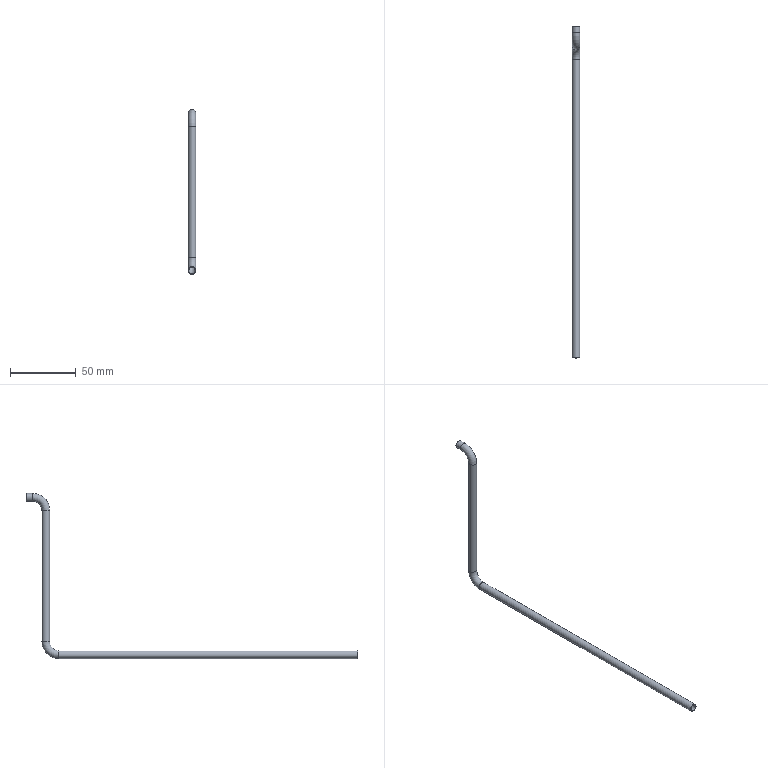Part | STEP file | 1-74 | 1 solid | 12 faces | box 6 x 253 x 126 mm | volume 3148 mm3 | cylinder 6 | torus 4 | plane 2 | commonest cylinder face diameters 5 x3 6 x3
STEP:
#1=CARTESIAN_POINT('',(0.,0.,0.));
#2=DIRECTION('',(0.,0.,1.));
#3=DIRECTION('',(1.,0.,0.));
#4=AXIS2_PLACEMENT_3D('',#1,#2,#3);
#5=CARTESIAN_POINT('',(3.,0.,0.));
#6=VERTEX_POINT('',#5);
#7=CARTESIAN_POINT('',(0.,0.,0.));
#8=DIRECTION('',(0.,-1.,0.));
#9=DIRECTION('',(1.,0.,0.));
#10=AXIS2_PLACEMENT_3D('',#7,#8,#9);
#11=CIRCLE('',#10,3.);
#12=CARTESIAN_POINT('',(0.,0.,0.));
#13=DIRECTION('',(0.,1.,0.));
#14=DIRECTION('',(1.,0.,0.));
#15=AXIS2_PLACEMENT_3D('',#12,#13,#14);
#16=CYLINDRICAL_SURFACE('',#15,3.);
#17=CARTESIAN_POINT('',(6.283,0.));
#18=DIRECTION('',(-1.,0.));
#19=VECTOR('',#18,1.);
#20=LINE('',#17,#19);
#21=(GEOMETRIC_REPRESENTATION_CONTEXT(2)PARAMETRIC_REPRESENTATION_CONTEXT()REPRESENTATION_CONTEXT('',''));
#22=DEFINITIONAL_REPRESENTATION('',(#20),#21);
#23=PCURVE('',#16,#22);
#24=CARTESIAN_POINT('',(0.,0.,0.));
#25=DIRECTION('',(0.,-1.,0.));
#26=DIRECTION('',(1.,0.,0.));
#27=AXIS2_PLACEMENT_3D('',#24,#25,#26);
#28=PLANE('',#27);
#29=CARTESIAN_POINT('',(0.,0.));
#30=DIRECTION('',(1.,0.));
#31=AXIS2_PLACEMENT_2D('',#29,#30);
#32=CIRCLE('',#31,3.);
#33=(GEOMETRIC_REPRESENTATION_CONTEXT(2)PARAMETRIC_REPRESENTATION_CONTEXT()REPRESENTATION_CONTEXT('',''));
#34=DEFINITIONAL_REPRESENTATION('',(#32),#33);
#35=PCURVE('',#28,#34);
#36=SURFACE_CURVE('',#11,(#23,#35),.PCURVE_S1.);
#37=EDGE_CURVE('',#6,#6,#36,.T.);
#38=ORIENTED_EDGE('',*,*,#37,.F.);
#39=CARTESIAN_POINT('',(3.,228.,0.));
#40=VERTEX_POINT('',#39);
#41=CARTESIAN_POINT('',(3.,0.,0.));
#42=DIRECTION('',(0.,1.,0.));
#43=VECTOR('',#42,1.);
#44=LINE('',#41,#43);
#45=CARTESIAN_POINT('',(6.283,0.));
#46=DIRECTION('',(0.,1.));
#47=VECTOR('',#46,1.);
#48=LINE('',#45,#47);
#49=(GEOMETRIC_REPRESENTATION_CONTEXT(2)PARAMETRIC_REPRESENTATION_CONTEXT()REPRESENTATION_CONTEXT('',''));
#50=DEFINITIONAL_REPRESENTATION('',(#48),#49);
#51=PCURVE('',#16,#50);
#52=CARTESIAN_POINT('',(0.,0.));
#53=DIRECTION('',(0.,1.));
#54=VECTOR('',#53,1.);
#55=LINE('',#52,#54);
#56=(GEOMETRIC_REPRESENTATION_CONTEXT(2)PARAMETRIC_REPRESENTATION_CONTEXT()REPRESENTATION_CONTEXT('',''));
#57=DEFINITIONAL_REPRESENTATION('',(#55),#56);
#58=PCURVE('',#16,#57);
#59=SEAM_CURVE('',#44,(#51,#58),.PCURVE_S1.);
#60=EDGE_CURVE('',#6,#40,#59,.T.);
#61=ORIENTED_EDGE('',*,*,#60,.T.);
#62=CARTESIAN_POINT('',(-3.,228.,0.));
#63=VERTEX_POINT('',#62);
#64=CARTESIAN_POINT('',(0.,228.,0.));
#65=DIRECTION('',(0.,1.,0.));
#66=DIRECTION('',(-1.,0.,0.));
#67=AXIS2_PLACEMENT_3D('',#64,#65,#66);
#68=CIRCLE('',#67,3.);
#69=CARTESIAN_POINT('',(3.142,228.));
#70=DIRECTION('',(1.,0.));
#71=VECTOR('',#70,1.);
#72=LINE('',#69,#71);
#73=(GEOMETRIC_REPRESENTATION_CONTEXT(2)PARAMETRIC_REPRESENTATION_CONTEXT()REPRESENTATION_CONTEXT('',''));
#74=DEFINITIONAL_REPRESENTATION('',(#72),#73);
#75=PCURVE('',#16,#74);
#76=CARTESIAN_POINT('',(0.,228.,10.));
#77=DIRECTION('',(-1.,0.,0.));
#78=DIRECTION('',(0.,0.,-1.));
#79=AXIS2_PLACEMENT_3D('',#76,#77,#78);
#80=TOROIDAL_SURFACE('',#79,10.,3.);
#81=CARTESIAN_POINT('',(6.283,1.571));
#82=CARTESIAN_POINT('',(6.283,1.618));
#83=CARTESIAN_POINT('',(6.283,1.714));
#84=CARTESIAN_POINT('',(6.283,1.856));
#85=CARTESIAN_POINT('',(6.283,1.999));
#86=CARTESIAN_POINT('',(6.283,2.142));
#87=CARTESIAN_POINT('',(6.283,2.285));
#88=CARTESIAN_POINT('',(6.283,2.428));
#89=CARTESIAN_POINT('',(6.283,2.57));
#90=CARTESIAN_POINT('',(6.283,2.713));
#91=CARTESIAN_POINT('',(6.283,2.856));
#92=CARTESIAN_POINT('',(6.283,2.999));
#93=CARTESIAN_POINT('',(6.283,3.142));
#94=CARTESIAN_POINT('',(6.283,3.284));
#95=CARTESIAN_POINT('',(6.283,3.427));
#96=CARTESIAN_POINT('',(6.283,3.57));
#97=CARTESIAN_POINT('',(6.283,3.713));
#98=CARTESIAN_POINT('',(6.283,3.856));
#99=CARTESIAN_POINT('',(6.283,3.998));
#100=CARTESIAN_POINT('',(6.283,4.141));
#101=CARTESIAN_POINT('',(6.283,4.284));
#102=CARTESIAN_POINT('',(6.283,4.427));
#103=CARTESIAN_POINT('',(6.283,4.57));
#104=CARTESIAN_POINT('',(6.283,4.665));
#105=CARTESIAN_POINT('',(6.283,4.712));
#106=B_SPLINE_CURVE_WITH_KNOTS('',3,(#81,#82,#83,#84,#85,#86,#87,#88,#89,#90,#91,#92,#93,#94,#95,#96,#97,#98,#99,#100,#101,#102,#103,#104,#105),.UNSPECIFIED.,.F.,.F.,(4,1,1,1,1,1,1,1,1,1,1,1,1,1,1,1,1,1,1,1,1,1,4),(0.,0.1428,0.2856,0.4284,0.5712,0.714,0.8568,0.9996,1.142,1.285,1.428,1.571,1.714,1.856,1.999,2.142,2.285,2.428,2.57,2.713,2.856,2.999,3.142),.QUASI_UNIFORM_KNOTS.);
#107=(GEOMETRIC_REPRESENTATION_CONTEXT(2)PARAMETRIC_REPRESENTATION_CONTEXT()REPRESENTATION_CONTEXT('',''));
#108=DEFINITIONAL_REPRESENTATION('',(#106),#107);
#109=PCURVE('',#80,#108);
#110=SURFACE_CURVE('',#68,(#75,#109),.PCURVE_S1.);
#111=EDGE_CURVE('',#63,#40,#110,.T.);
#112=ORIENTED_EDGE('',*,*,#111,.F.);
#113=CARTESIAN_POINT('',(0.,228.,0.));
#114=DIRECTION('',(0.,1.,0.));
#115=DIRECTION('',(1.,0.,0.));
#116=AXIS2_PLACEMENT_3D('',#113,#114,#115);
#117=CIRCLE('',#116,3.);
#118=CARTESIAN_POINT('',(0.,228.));
#119=DIRECTION('',(1.,0.));
#120=VECTOR('',#119,1.);
#121=LINE('',#118,#120);
#122=(GEOMETRIC_REPRESENTATION_CONTEXT(2)PARAMETRIC_REPRESENTATION_CONTEXT()REPRESENTATION_CONTEXT('',''));
#123=DEFINITIONAL_REPRESENTATION('',(#121),#122);
#124=PCURVE('',#16,#123);
#125=CARTESIAN_POINT('',(6.283,4.712));
#126=DIRECTION('',(0.,1.));
#127=VECTOR('',#126,1.);
#128=LINE('',#125,#127);
#129=(GEOMETRIC_REPRESENTATION_CONTEXT(2)PARAMETRIC_REPRESENTATION_CONTEXT()REPRESENTATION_CONTEXT('',''));
#130=DEFINITIONAL_REPRESENTATION('',(#128),#129);
#131=PCURVE('',#80,#130);
#132=SURFACE_CURVE('',#117,(#124,#131),.PCURVE_S1.);
#133=EDGE_CURVE('',#40,#63,#132,.T.);
#134=ORIENTED_EDGE('',*,*,#133,.F.);
#135=ORIENTED_EDGE('',*,*,#60,.F.);
#136=EDGE_LOOP('',(#38,#61,#112,#134,#135));
#137=FACE_BOUND('',#136,.T.);
#138=ADVANCED_FACE('',(#137),#16,.T.);
#139=ORIENTED_EDGE('',*,*,#111,.T.);
#140=ORIENTED_EDGE('',*,*,#133,.T.);
#141=CARTESIAN_POINT('',(-3.,238.,10.));
#142=VERTEX_POINT('',#141);
#143=CARTESIAN_POINT('',(-3.,228.,10.));
#144=DIRECTION('',(1.,0.,0.));
#145=DIRECTION('',(0.,0.,-1.));
#146=AXIS2_PLACEMENT_3D('',#143,#144,#145);
#147=CIRCLE('',#146,10.);
#148=CARTESIAN_POINT('',(6.283,7.854));
#149=DIRECTION('',(-1.,0.));
#150=VECTOR('',#149,1.);
#151=LINE('',#148,#150);
#152=(GEOMETRIC_REPRESENTATION_CONTEXT(2)PARAMETRIC_REPRESENTATION_CONTEXT()REPRESENTATION_CONTEXT('',''));
#153=DEFINITIONAL_REPRESENTATION('',(#151),#152);
#154=PCURVE('',#80,#153);
#155=CARTESIAN_POINT('',(6.283,1.571));
#156=DIRECTION('',(-1.,0.));
#157=VECTOR('',#156,1.);
#158=LINE('',#155,#157);
#159=(GEOMETRIC_REPRESENTATION_CONTEXT(2)PARAMETRIC_REPRESENTATION_CONTEXT()REPRESENTATION_CONTEXT('',''));
#160=DEFINITIONAL_REPRESENTATION('',(#158),#159);
#161=PCURVE('',#80,#160);
#162=SEAM_CURVE('',#147,(#154,#161),.PCURVE_S1.);
#163=EDGE_CURVE('',#63,#142,#162,.T.);
#164=ORIENTED_EDGE('',*,*,#163,.T.);
#165=CARTESIAN_POINT('',(3.,238.,10.));
#166=VERTEX_POINT('',#165);
#167=CARTESIAN_POINT('',(0.,238.,10.));
#168=DIRECTION('',(0.,0.,-1.));
#169=DIRECTION('',(-1.,0.,0.));
#170=AXIS2_PLACEMENT_3D('',#167,#168,#169);
#171=CIRCLE('',#170,3.);
#172=CARTESIAN_POINT('',(4.712,7.854));
#173=DIRECTION('',(0.,-1.));
#174=VECTOR('',#173,1.);
#175=LINE('',#172,#174);
#176=(GEOMETRIC_REPRESENTATION_CONTEXT(2)PARAMETRIC_REPRESENTATION_CONTEXT()REPRESENTATION_CONTEXT('',''));
#177=DEFINITIONAL_REPRESENTATION('',(#175),#176);
#178=PCURVE('',#80,#177);
#179=CARTESIAN_POINT('',(0.,238.,10.));
#180=DIRECTION('',(0.,0.,1.));
#181=DIRECTION('',(1.,0.,0.));
#182=AXIS2_PLACEMENT_3D('',#179,#180,#181);
#183=CYLINDRICAL_SURFACE('',#182,3.);
#184=CARTESIAN_POINT('',(3.142,0.));
#185=DIRECTION('',(-1.,0.));
#186=VECTOR('',#185,1.);
#187=LINE('',#184,#186);
#188=(GEOMETRIC_REPRESENTATION_CONTEXT(2)PARAMETRIC_REPRESENTATION_CONTEXT()REPRESENTATION_CONTEXT('',''));
#189=DEFINITIONAL_REPRESENTATION('',(#187),#188);
#190=PCURVE('',#183,#189);
#191=SURFACE_CURVE('',#171,(#178,#190),.PCURVE_S1.);
#192=EDGE_CURVE('',#142,#166,#191,.T.);
#193=ORIENTED_EDGE('',*,*,#192,.T.);
#194=CARTESIAN_POINT('',(0.,238.,10.));
#195=DIRECTION('',(0.,0.,-1.));
#196=DIRECTION('',(1.,0.,0.));
#197=AXIS2_PLACEMENT_3D('',#194,#195,#196);
#198=CIRCLE('',#197,3.);
#199=CARTESIAN_POINT('',(4.712,4.712));
#200=DIRECTION('',(0.,-1.));
#201=VECTOR('',#200,1.);
#202=LINE('',#199,#201);
#203=(GEOMETRIC_REPRESENTATION_CONTEXT(2)PARAMETRIC_REPRESENTATION_CONTEXT()REPRESENTATION_CONTEXT('',''));
#204=DEFINITIONAL_REPRESENTATION('',(#202),#203);
#205=PCURVE('',#80,#204);
#206=CARTESIAN_POINT('',(6.283,0.));
#207=DIRECTION('',(-1.,0.));
#208=VECTOR('',#207,1.);
#209=LINE('',#206,#208);
#210=(GEOMETRIC_REPRESENTATION_CONTEXT(2)PARAMETRIC_REPRESENTATION_CONTEXT()REPRESENTATION_CONTEXT('',''));
#211=DEFINITIONAL_REPRESENTATION('',(#209),#210);
#212=PCURVE('',#183,#211);
#213=SURFACE_CURVE('',#198,(#205,#212),.PCURVE_S1.);
#214=EDGE_CURVE('',#166,#142,#213,.T.);
#215=ORIENTED_EDGE('',*,*,#214,.T.);
#216=ORIENTED_EDGE('',*,*,#163,.F.);
#217=EDGE_LOOP('',(#139,#140,#164,#193,#215,#216));
#218=FACE_BOUND('',#217,.T.);
#219=ADVANCED_FACE('',(#218),#80,.T.);
#220=ORIENTED_EDGE('',*,*,#192,.F.);
#221=ORIENTED_EDGE('',*,*,#214,.F.);
#222=CARTESIAN_POINT('',(3.,238.,110.));
#223=VERTEX_POINT('',#222);
#224=CARTESIAN_POINT('',(3.,238.,10.));
#225=DIRECTION('',(0.,0.,1.));
#226=VECTOR('',#225,1.);
#227=LINE('',#224,#226);
#228=CARTESIAN_POINT('',(6.283,0.));
#229=DIRECTION('',(0.,1.));
#230=VECTOR('',#229,1.);
#231=LINE('',#228,#230);
#232=(GEOMETRIC_REPRESENTATION_CONTEXT(2)PARAMETRIC_REPRESENTATION_CONTEXT()REPRESENTATION_CONTEXT('',''));
#233=DEFINITIONAL_REPRESENTATION('',(#231),#232);
#234=PCURVE('',#183,#233);
#235=CARTESIAN_POINT('',(0.,0.));
#236=DIRECTION('',(0.,1.));
#237=VECTOR('',#236,1.);
#238=LINE('',#235,#237);
#239=(GEOMETRIC_REPRESENTATION_CONTEXT(2)PARAMETRIC_REPRESENTATION_CONTEXT()REPRESENTATION_CONTEXT('',''));
#240=DEFINITIONAL_REPRESENTATION('',(#238),#239);
#241=PCURVE('',#183,#240);
#242=SEAM_CURVE('',#227,(#234,#241),.PCURVE_S1.);
#243=EDGE_CURVE('',#166,#223,#242,.T.);
#244=ORIENTED_EDGE('',*,*,#243,.T.);
#245=CARTESIAN_POINT('',(-3.,238.,110.));
#246=VERTEX_POINT('',#245);
#247=CARTESIAN_POINT('',(0.,238.,110.));
#248=DIRECTION('',(0.,0.,1.));
#249=DIRECTION('',(-1.,0.,0.));
#250=AXIS2_PLACEMENT_3D('',#247,#248,#249);
#251=CIRCLE('',#250,3.);
#252=CARTESIAN_POINT('',(3.142,100.));
#253=DIRECTION('',(1.,0.));
#254=VECTOR('',#253,1.);
#255=LINE('',#252,#254);
#256=(GEOMETRIC_REPRESENTATION_CONTEXT(2)PARAMETRIC_REPRESENTATION_CONTEXT()REPRESENTATION_CONTEXT('',''));
#257=DEFINITIONAL_REPRESENTATION('',(#255),#256);
#258=PCURVE('',#183,#257);
#259=CARTESIAN_POINT('',(0.,248.,110.));
#260=DIRECTION('',(1.,0.,0.));
#261=DIRECTION('',(0.,-1.,0.));
#262=AXIS2_PLACEMENT_3D('',#259,#260,#261);
#263=TOROIDAL_SURFACE('',#262,10.,3.);
#264=CARTESIAN_POINT('',(6.283,-1.571));
#265=DIRECTION('',(0.,1.));
#266=VECTOR('',#265,1.);
#267=LINE('',#264,#266);
#268=(GEOMETRIC_REPRESENTATION_CONTEXT(2)PARAMETRIC_REPRESENTATION_CONTEXT()REPRESENTATION_CONTEXT('',''));
#269=DEFINITIONAL_REPRESENTATION('',(#267),#268);
#270=PCURVE('',#263,#269);
#271=SURFACE_CURVE('',#251,(#258,#270),.PCURVE_S1.);
#272=EDGE_CURVE('',#246,#223,#271,.T.);
#273=ORIENTED_EDGE('',*,*,#272,.F.);
#274=CARTESIAN_POINT('',(0.,238.,110.));
#275=DIRECTION('',(0.,0.,1.));
#276=DIRECTION('',(1.,0.,0.));
#277=AXIS2_PLACEMENT_3D('',#274,#275,#276);
#278=CIRCLE('',#277,3.);
#279=CARTESIAN_POINT('',(0.,100.));
#280=DIRECTION('',(1.,0.));
#281=VECTOR('',#280,1.);
#282=LINE('',#279,#281);
#283=(GEOMETRIC_REPRESENTATION_CONTEXT(2)PARAMETRIC_REPRESENTATION_CONTEXT()REPRESENTATION_CONTEXT('',''));
#284=DEFINITIONAL_REPRESENTATION('',(#282),#283);
#285=PCURVE('',#183,#284);
#286=CARTESIAN_POINT('',(6.283,1.571));
#287=DIRECTION('',(0.,1.));
#288=VECTOR('',#287,1.);
#289=LINE('',#286,#288);
#290=(GEOMETRIC_REPRESENTATION_CONTEXT(2)PARAMETRIC_REPRESENTATION_CONTEXT()REPRESENTATION_CONTEXT('',''));
#291=DEFINITIONAL_REPRESENTATION('',(#289),#290);
#292=PCURVE('',#263,#291);
#293=SURFACE_CURVE('',#278,(#285,#292),.PCURVE_S1.);
#294=EDGE_CURVE('',#223,#246,#293,.T.);
#295=ORIENTED_EDGE('',*,*,#294,.F.);
#296=ORIENTED_EDGE('',*,*,#243,.F.);
#297=EDGE_LOOP('',(#220,#221,#244,#273,#295,#296));
#298=FACE_BOUND('',#297,.T.);
#299=ADVANCED_FACE('',(#298),#183,.T.);
#300=ORIENTED_EDGE('',*,*,#272,.T.);
#301=ORIENTED_EDGE('',*,*,#294,.T.);
#302=CARTESIAN_POINT('',(-3.,248.,120.));
#303=VERTEX_POINT('',#302);
#304=CARTESIAN_POINT('',(-3.,248.,110.));
#305=DIRECTION('',(-1.,0.,0.));
#306=DIRECTION('',(0.,-1.,0.));
#307=AXIS2_PLACEMENT_3D('',#304,#305,#306);
#308=CIRCLE('',#307,10.);
#309=CARTESIAN_POINT('',(6.283,4.712));
#310=DIRECTION('',(-1.,0.));
#311=VECTOR('',#310,1.);
#312=LINE('',#309,#311);
#313=(GEOMETRIC_REPRESENTATION_CONTEXT(2)PARAMETRIC_REPRESENTATION_CONTEXT()REPRESENTATION_CONTEXT('',''));
#314=DEFINITIONAL_REPRESENTATION('',(#312),#313);
#315=PCURVE('',#263,#314);
#316=CARTESIAN_POINT('',(6.283,-1.571));
#317=DIRECTION('',(-1.,0.));
#318=VECTOR('',#317,1.);
#319=LINE('',#316,#318);
#320=(GEOMETRIC_REPRESENTATION_CONTEXT(2)PARAMETRIC_REPRESENTATION_CONTEXT()REPRESENTATION_CONTEXT('',''));
#321=DEFINITIONAL_REPRESENTATION('',(#319),#320);
#322=PCURVE('',#263,#321);
#323=SEAM_CURVE('',#308,(#315,#322),.PCURVE_S1.);
#324=EDGE_CURVE('',#246,#303,#323,.T.);
#325=ORIENTED_EDGE('',*,*,#324,.T.);
#326=CARTESIAN_POINT('',(3.,248.,120.));
#327=VERTEX_POINT('',#326);
#328=CARTESIAN_POINT('',(0.,248.,120.));
#329=DIRECTION('',(0.,-1.,0.));
#330=DIRECTION('',(-1.,0.,0.));
#331=AXIS2_PLACEMENT_3D('',#328,#329,#330);
#332=CIRCLE('',#331,3.);
#333=CARTESIAN_POINT('',(4.712,4.712));
#334=DIRECTION('',(0.,-1.));
#335=VECTOR('',#334,1.);
#336=LINE('',#333,#335);
#337=(GEOMETRIC_REPRESENTATION_CONTEXT(2)PARAMETRIC_REPRESENTATION_CONTEXT()REPRESENTATION_CONTEXT('',''));
#338=DEFINITIONAL_REPRESENTATION('',(#336),#337);
#339=PCURVE('',#263,#338);
#340=CARTESIAN_POINT('',(0.,248.,120.));
#341=DIRECTION('',(0.,1.,0.));
#342=DIRECTION('',(1.,0.,0.));
#343=AXIS2_PLACEMENT_3D('',#340,#341,#342);
#344=CYLINDRICAL_SURFACE('',#343,3.);
#345=CARTESIAN_POINT('',(3.142,0.));
#346=DIRECTION('',(-1.,0.));
#347=VECTOR('',#346,1.);
#348=LINE('',#345,#347);
#349=(GEOMETRIC_REPRESENTATION_CONTEXT(2)PARAMETRIC_REPRESENTATION_CONTEXT()REPRESENTATION_CONTEXT('',''));
#350=DEFINITIONAL_REPRESENTATION('',(#348),#349);
#351=PCURVE('',#344,#350);
#352=SURFACE_CURVE('',#332,(#339,#351),.PCURVE_S1.);
#353=EDGE_CURVE('',#303,#327,#352,.T.);
#354=ORIENTED_EDGE('',*,*,#353,.T.);
#355=CARTESIAN_POINT('',(0.,248.,120.));
#356=DIRECTION('',(0.,-1.,0.));
#357=DIRECTION('',(1.,0.,0.));
#358=AXIS2_PLACEMENT_3D('',#355,#356,#357);
#359=CIRCLE('',#358,3.);
#360=CARTESIAN_POINT('',(4.712,1.571));
#361=DIRECTION('',(0.,-1.));
#362=VECTOR('',#361,1.);
#363=LINE('',#360,#362);
#364=(GEOMETRIC_REPRESENTATION_CONTEXT(2)PARAMETRIC_REPRESENTATION_CONTEXT()REPRESENTATION_CONTEXT('',''));
#365=DEFINITIONAL_REPRESENTATION('',(#363),#364);
#366=PCURVE('',#263,#365);
#367=CARTESIAN_POINT('',(6.283,0.));
#368=DIRECTION('',(-1.,0.));
#369=VECTOR('',#368,1.);
#370=LINE('',#367,#369);
#371=(GEOMETRIC_REPRESENTATION_CONTEXT(2)PARAMETRIC_REPRESENTATION_CONTEXT()REPRESENTATION_CONTEXT('',''));
#372=DEFINITIONAL_REPRESENTATION('',(#370),#371);
#373=PCURVE('',#344,#372);
#374=SURFACE_CURVE('',#359,(#366,#373),.PCURVE_S1.);
#375=EDGE_CURVE('',#327,#303,#374,.T.);
#376=ORIENTED_EDGE('',*,*,#375,.T.);
#377=ORIENTED_EDGE('',*,*,#324,.F.);
#378=EDGE_LOOP('',(#300,#301,#325,#354,#376,#377));
#379=FACE_BOUND('',#378,.T.);
#380=ADVANCED_FACE('',(#379),#263,.T.);
#381=ORIENTED_EDGE('',*,*,#353,.F.);
#382=ORIENTED_EDGE('',*,*,#375,.F.);
#383=CARTESIAN_POINT('',(3.,253.,120.));
#384=VERTEX_POINT('',#383);
#385=CARTESIAN_POINT('',(3.,248.,120.));
#386=DIRECTION('',(0.,1.,0.));
#387=VECTOR('',#386,1.);
#388=LINE('',#385,#387);
#389=CARTESIAN_POINT('',(6.283,0.));
#390=DIRECTION('',(0.,1.));
#391=VECTOR('',#390,1.);
#392=LINE('',#389,#391);
#393=(GEOMETRIC_REPRESENTATION_CONTEXT(2)PARAMETRIC_REPRESENTATION_CONTEXT()REPRESENTATION_CONTEXT('',''));
#394=DEFINITIONAL_REPRESENTATION('',(#392),#393);
#395=PCURVE('',#344,#394);
#396=CARTESIAN_POINT('',(0.,0.));
#397=DIRECTION('',(0.,1.));
#398=VECTOR('',#397,1.);
#399=LINE('',#396,#398);
#400=(GEOMETRIC_REPRESENTATION_CONTEXT(2)PARAMETRIC_REPRESENTATION_CONTEXT()REPRESENTATION_CONTEXT('',''));
#401=DEFINITIONAL_REPRESENTATION('',(#399),#400);
#402=PCURVE('',#344,#401);
#403=SEAM_CURVE('',#388,(#395,#402),.PCURVE_S1.);
#404=EDGE_CURVE('',#327,#384,#403,.T.);
#405=ORIENTED_EDGE('',*,*,#404,.T.);
#406=CARTESIAN_POINT('',(0.,253.,120.));
#407=DIRECTION('',(0.,1.,0.));
#408=DIRECTION('',(1.,0.,0.));
#409=AXIS2_PLACEMENT_3D('',#406,#407,#408);
#410=CIRCLE('',#409,3.);
#411=CARTESIAN_POINT('',(0.,5.));
#412=DIRECTION('',(1.,0.));
#413=VECTOR('',#412,1.);
#414=LINE('',#411,#413);
#415=(GEOMETRIC_REPRESENTATION_CONTEXT(2)PARAMETRIC_REPRESENTATION_CONTEXT()REPRESENTATION_CONTEXT('',''));
#416=DEFINITIONAL_REPRESENTATION('',(#414),#415);
#417=PCURVE('',#344,#416);
#418=CARTESIAN_POINT('',(0.,253.,120.));
#419=DIRECTION('',(0.,1.,0.));
#420=DIRECTION('',(0.,0.,1.));
#421=AXIS2_PLACEMENT_3D('',#418,#419,#420);
#422=PLANE('',#421);
#423=CARTESIAN_POINT('',(0.,0.));
#424=DIRECTION('',(0.,1.));
#425=AXIS2_PLACEMENT_2D('',#423,#424);
#426=CIRCLE('',#425,3.);
#427=(GEOMETRIC_REPRESENTATION_CONTEXT(2)PARAMETRIC_REPRESENTATION_CONTEXT()REPRESENTATION_CONTEXT('',''));
#428=DEFINITIONAL_REPRESENTATION('',(#426),#427);
#429=PCURVE('',#422,#428);
#430=SURFACE_CURVE('',#410,(#417,#429),.PCURVE_S1.);
#431=EDGE_CURVE('',#384,#384,#430,.T.);
#432=ORIENTED_EDGE('',*,*,#431,.F.);
#433=ORIENTED_EDGE('',*,*,#404,.F.);
#434=EDGE_LOOP('',(#381,#382,#405,#432,#433));
#435=FACE_BOUND('',#434,.T.);
#436=ADVANCED_FACE('',(#435),#344,.T.);
#437=ORIENTED_EDGE('',*,*,#37,.T.);
#438=EDGE_LOOP('',(#437));
#439=FACE_BOUND('',#438,.T.);
#440=CARTESIAN_POINT('',(2.5,0.,0.));
#441=VERTEX_POINT('',#440);
#442=CARTESIAN_POINT('',(0.,0.,0.));
#443=DIRECTION('',(0.,-1.,0.));
#444=DIRECTION('',(1.,0.,0.));
#445=AXIS2_PLACEMENT_3D('',#442,#443,#444);
#446=CIRCLE('',#445,2.5);
#447=CARTESIAN_POINT('',(0.,0.));
#448=DIRECTION('',(1.,0.));
#449=AXIS2_PLACEMENT_2D('',#447,#448);
#450=CIRCLE('',#449,2.5);
#451=(GEOMETRIC_REPRESENTATION_CONTEXT(2)PARAMETRIC_REPRESENTATION_CONTEXT()REPRESENTATION_CONTEXT('',''));
#452=DEFINITIONAL_REPRESENTATION('',(#450),#451);
#453=PCURVE('',#28,#452);
#454=CARTESIAN_POINT('',(0.,0.,0.));
#455=DIRECTION('',(0.,1.,0.));
#456=DIRECTION('',(1.,0.,0.));
#457=AXIS2_PLACEMENT_3D('',#454,#455,#456);
#458=CYLINDRICAL_SURFACE('',#457,2.5);
#459=CARTESIAN_POINT('',(6.283,0.));
#460=DIRECTION('',(-1.,0.));
#461=VECTOR('',#460,1.);
#462=LINE('',#459,#461);
#463=(GEOMETRIC_REPRESENTATION_CONTEXT(2)PARAMETRIC_REPRESENTATION_CONTEXT()REPRESENTATION_CONTEXT('',''));
#464=DEFINITIONAL_REPRESENTATION('',(#462),#463);
#465=PCURVE('',#458,#464);
#466=SURFACE_CURVE('',#446,(#453,#465),.PCURVE_S1.);
#467=EDGE_CURVE('',#441,#441,#466,.T.);
#468=ORIENTED_EDGE('',*,*,#467,.F.);
#469=EDGE_LOOP('',(#468));
#470=FACE_BOUND('',#469,.T.);
#471=ADVANCED_FACE('',(#439,#470),#28,.T.);
#472=ORIENTED_EDGE('',*,*,#431,.T.);
#473=EDGE_LOOP('',(#472));
#474=FACE_BOUND('',#473,.T.);
#475=CARTESIAN_POINT('',(2.5,253.,120.));
#476=VERTEX_POINT('',#475);
#477=CARTESIAN_POINT('',(0.,253.,120.));
#478=DIRECTION('',(0.,1.,0.));
#479=DIRECTION('',(1.,0.,0.));
#480=AXIS2_PLACEMENT_3D('',#477,#478,#479);
#481=CIRCLE('',#480,2.5);
#482=CARTESIAN_POINT('',(0.,0.));
#483=DIRECTION('',(0.,1.));
#484=AXIS2_PLACEMENT_2D('',#482,#483);
#485=CIRCLE('',#484,2.5);
#486=(GEOMETRIC_REPRESENTATION_CONTEXT(2)PARAMETRIC_REPRESENTATION_CONTEXT()REPRESENTATION_CONTEXT('',''));
#487=DEFINITIONAL_REPRESENTATION('',(#485),#486);
#488=PCURVE('',#422,#487);
#489=CARTESIAN_POINT('',(0.,248.,120.));
#490=DIRECTION('',(0.,1.,0.));
#491=DIRECTION('',(1.,0.,0.));
#492=AXIS2_PLACEMENT_3D('',#489,#490,#491);
#493=CYLINDRICAL_SURFACE('',#492,2.5);
#494=CARTESIAN_POINT('',(0.,5.));
#495=DIRECTION('',(1.,0.));
#496=VECTOR('',#495,1.);
#497=LINE('',#494,#496);
#498=(GEOMETRIC_REPRESENTATION_CONTEXT(2)PARAMETRIC_REPRESENTATION_CONTEXT()REPRESENTATION_CONTEXT('',''));
#499=DEFINITIONAL_REPRESENTATION('',(#497),#498);
#500=PCURVE('',#493,#499);
#501=SURFACE_CURVE('',#481,(#488,#500),.PCURVE_S1.);
#502=EDGE_CURVE('',#476,#476,#501,.T.);
#503=ORIENTED_EDGE('',*,*,#502,.F.);
#504=EDGE_LOOP('',(#503));
#505=FACE_BOUND('',#504,.T.);
#506=ADVANCED_FACE('',(#474,#505),#422,.T.);
#507=ORIENTED_EDGE('',*,*,#467,.F.);
#508=CARTESIAN_POINT('',(2.5,228.,0.));
#509=VERTEX_POINT('',#508);
#510=CARTESIAN_POINT('',(2.5,0.,0.));
#511=DIRECTION('',(0.,1.,0.));
#512=VECTOR('',#511,1.);
#513=LINE('',#510,#512);
#514=CARTESIAN_POINT('',(6.283,0.));
#515=DIRECTION('',(0.,1.));
#516=VECTOR('',#515,1.);
#517=LINE('',#514,#516);
#518=(GEOMETRIC_REPRESENTATION_CONTEXT(2)PARAMETRIC_REPRESENTATION_CONTEXT()REPRESENTATION_CONTEXT('',''));
#519=DEFINITIONAL_REPRESENTATION('',(#517),#518);
#520=PCURVE('',#458,#519);
#521=CARTESIAN_POINT('',(0.,0.));
#522=DIRECTION('',(0.,1.));
#523=VECTOR('',#522,1.);
#524=LINE('',#521,#523);
#525=(GEOMETRIC_REPRESENTATION_CONTEXT(2)PARAMETRIC_REPRESENTATION_CONTEXT()REPRESENTATION_CONTEXT('',''));
#526=DEFINITIONAL_REPRESENTATION('',(#524),#525);
#527=PCURVE('',#458,#526);
#528=SEAM_CURVE('',#513,(#520,#527),.PCURVE_S1.);
#529=EDGE_CURVE('',#441,#509,#528,.T.);
#530=ORIENTED_EDGE('',*,*,#529,.T.);
#531=CARTESIAN_POINT('',(-2.5,228.,0.));
#532=VERTEX_POINT('',#531);
#533=CARTESIAN_POINT('',(0.,228.,0.));
#534=DIRECTION('',(0.,1.,0.));
#535=DIRECTION('',(-1.,0.,0.));
#536=AXIS2_PLACEMENT_3D('',#533,#534,#535);
#537=CIRCLE('',#536,2.5);
#538=CARTESIAN_POINT('',(3.142,228.));
#539=DIRECTION('',(1.,0.));
#540=VECTOR('',#539,1.);
#541=LINE('',#538,#540);
#542=(GEOMETRIC_REPRESENTATION_CONTEXT(2)PARAMETRIC_REPRESENTATION_CONTEXT()REPRESENTATION_CONTEXT('',''));
#543=DEFINITIONAL_REPRESENTATION('',(#541),#542);
#544=PCURVE('',#458,#543);
#545=CARTESIAN_POINT('',(0.,228.,10.));
#546=DIRECTION('',(-1.,0.,0.));
#547=DIRECTION('',(0.,0.,-1.));
#548=AXIS2_PLACEMENT_3D('',#545,#546,#547);
#549=TOROIDAL_SURFACE('',#548,10.,2.5);
#550=CARTESIAN_POINT('',(6.283,1.571));
#551=DIRECTION('',(0.,1.));
#552=VECTOR('',#551,1.);
#553=LINE('',#550,#552);
#554=(GEOMETRIC_REPRESENTATION_CONTEXT(2)PARAMETRIC_REPRESENTATION_CONTEXT()REPRESENTATION_CONTEXT('',''));
#555=DEFINITIONAL_REPRESENTATION('',(#553),#554);
#556=PCURVE('',#549,#555);
#557=SURFACE_CURVE('',#537,(#544,#556),.PCURVE_S1.);
#558=EDGE_CURVE('',#532,#509,#557,.T.);
#559=ORIENTED_EDGE('',*,*,#558,.F.);
#560=CARTESIAN_POINT('',(0.,228.,0.));
#561=DIRECTION('',(0.,1.,0.));
#562=DIRECTION('',(1.,0.,0.));
#563=AXIS2_PLACEMENT_3D('',#560,#561,#562);
#564=CIRCLE('',#563,2.5);
#565=CARTESIAN_POINT('',(0.,228.));
#566=DIRECTION('',(1.,0.));
#567=VECTOR('',#566,1.);
#568=LINE('',#565,#567);
#569=(GEOMETRIC_REPRESENTATION_CONTEXT(2)PARAMETRIC_REPRESENTATION_CONTEXT()REPRESENTATION_CONTEXT('',''));
#570=DEFINITIONAL_REPRESENTATION('',(#568),#569);
#571=PCURVE('',#458,#570);
#572=CARTESIAN_POINT('',(6.283,4.712));
#573=DIRECTION('',(0.,1.));
#574=VECTOR('',#573,1.);
#575=LINE('',#572,#574);
#576=(GEOMETRIC_REPRESENTATION_CONTEXT(2)PARAMETRIC_REPRESENTATION_CONTEXT()REPRESENTATION_CONTEXT('',''));
#577=DEFINITIONAL_REPRESENTATION('',(#575),#576);
#578=PCURVE('',#549,#577);
#579=SURFACE_CURVE('',#564,(#571,#578),.PCURVE_S1.);
#580=EDGE_CURVE('',#509,#532,#579,.T.);
#581=ORIENTED_EDGE('',*,*,#580,.F.);
#582=ORIENTED_EDGE('',*,*,#529,.F.);
#583=EDGE_LOOP('',(#507,#530,#559,#581,#582));
#584=FACE_BOUND('',#583,.F.);
#585=ADVANCED_FACE('',(#584),#458,.F.);
#586=ORIENTED_EDGE('',*,*,#558,.T.);
#587=ORIENTED_EDGE('',*,*,#580,.T.);
#588=CARTESIAN_POINT('',(-2.5,238.,10.));
#589=VERTEX_POINT('',#588);
#590=CARTESIAN_POINT('',(-2.5,228.,10.));
#591=DIRECTION('',(1.,0.,0.));
#592=DIRECTION('',(0.,0.,-1.));
#593=AXIS2_PLACEMENT_3D('',#590,#591,#592);
#594=CIRCLE('',#593,10.);
#595=CARTESIAN_POINT('',(6.283,7.854));
#596=DIRECTION('',(-1.,0.));
#597=VECTOR('',#596,1.);
#598=LINE('',#595,#597);
#599=(GEOMETRIC_REPRESENTATION_CONTEXT(2)PARAMETRIC_REPRESENTATION_CONTEXT()REPRESENTATION_CONTEXT('',''));
#600=DEFINITIONAL_REPRESENTATION('',(#598),#599);
#601=PCURVE('',#549,#600);
#602=CARTESIAN_POINT('',(6.283,1.571));
#603=DIRECTION('',(-1.,0.));
#604=VECTOR('',#603,1.);
#605=LINE('',#602,#604);
#606=(GEOMETRIC_REPRESENTATION_CONTEXT(2)PARAMETRIC_REPRESENTATION_CONTEXT()REPRESENTATION_CONTEXT('',''));
#607=DEFINITIONAL_REPRESENTATION('',(#605),#606);
#608=PCURVE('',#549,#607);
#609=SEAM_CURVE('',#594,(#601,#608),.PCURVE_S1.);
#610=EDGE_CURVE('',#532,#589,#609,.T.);
#611=ORIENTED_EDGE('',*,*,#610,.T.);
#612=CARTESIAN_POINT('',(2.5,238.,10.));
#613=VERTEX_POINT('',#612);
#614=CARTESIAN_POINT('',(0.,238.,10.));
#615=DIRECTION('',(0.,0.,-1.));
#616=DIRECTION('',(-1.,0.,0.));
#617=AXIS2_PLACEMENT_3D('',#614,#615,#616);
#618=CIRCLE('',#617,2.5);
#619=CARTESIAN_POINT('',(4.712,7.854));
#620=DIRECTION('',(0.,-1.));
#621=VECTOR('',#620,1.);
#622=LINE('',#619,#621);
#623=(GEOMETRIC_REPRESENTATION_CONTEXT(2)PARAMETRIC_REPRESENTATION_CONTEXT()REPRESENTATION_CONTEXT('',''));
#624=DEFINITIONAL_REPRESENTATION('',(#622),#623);
#625=PCURVE('',#549,#624);
#626=CARTESIAN_POINT('',(0.,238.,10.));
#627=DIRECTION('',(0.,0.,1.));
#628=DIRECTION('',(1.,0.,0.));
#629=AXIS2_PLACEMENT_3D('',#626,#627,#628);
#630=CYLINDRICAL_SURFACE('',#629,2.5);
#631=CARTESIAN_POINT('',(3.142,0.));
#632=DIRECTION('',(-1.,0.));
#633=VECTOR('',#632,1.);
#634=LINE('',#631,#633);
#635=(GEOMETRIC_REPRESENTATION_CONTEXT(2)PARAMETRIC_REPRESENTATION_CONTEXT()REPRESENTATION_CONTEXT('',''));
#636=DEFINITIONAL_REPRESENTATION('',(#634),#635);
#637=PCURVE('',#630,#636);
#638=SURFACE_CURVE('',#618,(#625,#637),.PCURVE_S1.);
#639=EDGE_CURVE('',#589,#613,#638,.T.);
#640=ORIENTED_EDGE('',*,*,#639,.T.);
#641=CARTESIAN_POINT('',(0.,238.,10.));
#642=DIRECTION('',(0.,0.,-1.));
#643=DIRECTION('',(1.,0.,0.));
#644=AXIS2_PLACEMENT_3D('',#641,#642,#643);
#645=CIRCLE('',#644,2.5);
#646=CARTESIAN_POINT('',(4.712,4.712));
#647=DIRECTION('',(0.,-1.));
#648=VECTOR('',#647,1.);
#649=LINE('',#646,#648);
#650=(GEOMETRIC_REPRESENTATION_CONTEXT(2)PARAMETRIC_REPRESENTATION_CONTEXT()REPRESENTATION_CONTEXT('',''));
#651=DEFINITIONAL_REPRESENTATION('',(#649),#650);
#652=PCURVE('',#549,#651);
#653=CARTESIAN_POINT('',(6.283,0.));
#654=DIRECTION('',(-1.,0.));
#655=VECTOR('',#654,1.);
#656=LINE('',#653,#655);
#657=(GEOMETRIC_REPRESENTATION_CONTEXT(2)PARAMETRIC_REPRESENTATION_CONTEXT()REPRESENTATION_CONTEXT('',''));
#658=DEFINITIONAL_REPRESENTATION('',(#656),#657);
#659=PCURVE('',#630,#658);
#660=SURFACE_CURVE('',#645,(#652,#659),.PCURVE_S1.);
#661=EDGE_CURVE('',#613,#589,#660,.T.);
#662=ORIENTED_EDGE('',*,*,#661,.T.);
#663=ORIENTED_EDGE('',*,*,#610,.F.);
#664=EDGE_LOOP('',(#586,#587,#611,#640,#662,#663));
#665=FACE_BOUND('',#664,.F.);
#666=ADVANCED_FACE('',(#665),#549,.F.);
#667=ORIENTED_EDGE('',*,*,#639,.F.);
#668=ORIENTED_EDGE('',*,*,#661,.F.);
#669=CARTESIAN_POINT('',(2.5,238.,110.));
#670=VERTEX_POINT('',#669);
#671=CARTESIAN_POINT('',(2.5,238.,10.));
#672=DIRECTION('',(0.,0.,1.));
#673=VECTOR('',#672,1.);
#674=LINE('',#671,#673);
#675=CARTESIAN_POINT('',(6.283,0.));
#676=DIRECTION('',(0.,1.));
#677=VECTOR('',#676,1.);
#678=LINE('',#675,#677);
#679=(GEOMETRIC_REPRESENTATION_CONTEXT(2)PARAMETRIC_REPRESENTATION_CONTEXT()REPRESENTATION_CONTEXT('',''));
#680=DEFINITIONAL_REPRESENTATION('',(#678),#679);
#681=PCURVE('',#630,#680);
#682=CARTESIAN_POINT('',(0.,0.));
#683=DIRECTION('',(0.,1.));
#684=VECTOR('',#683,1.);
#685=LINE('',#682,#684);
#686=(GEOMETRIC_REPRESENTATION_CONTEXT(2)PARAMETRIC_REPRESENTATION_CONTEXT()REPRESENTATION_CONTEXT('',''));
#687=DEFINITIONAL_REPRESENTATION('',(#685),#686);
#688=PCURVE('',#630,#687);
#689=SEAM_CURVE('',#674,(#681,#688),.PCURVE_S1.);
#690=EDGE_CURVE('',#613,#670,#689,.T.);
#691=ORIENTED_EDGE('',*,*,#690,.T.);
#692=CARTESIAN_POINT('',(-2.5,238.,110.));
#693=VERTEX_POINT('',#692);
#694=CARTESIAN_POINT('',(0.,238.,110.));
#695=DIRECTION('',(0.,0.,1.));
#696=DIRECTION('',(-1.,0.,0.));
#697=AXIS2_PLACEMENT_3D('',#694,#695,#696);
#698=CIRCLE('',#697,2.5);
#699=CARTESIAN_POINT('',(3.142,100.));
#700=DIRECTION('',(1.,0.));
#701=VECTOR('',#700,1.);
#702=LINE('',#699,#701);
#703=(GEOMETRIC_REPRESENTATION_CONTEXT(2)PARAMETRIC_REPRESENTATION_CONTEXT()REPRESENTATION_CONTEXT('',''));
#704=DEFINITIONAL_REPRESENTATION('',(#702),#703);
#705=PCURVE('',#630,#704);
#706=CARTESIAN_POINT('',(0.,248.,110.));
#707=DIRECTION('',(1.,0.,0.));
#708=DIRECTION('',(0.,-1.,0.));
#709=AXIS2_PLACEMENT_3D('',#706,#707,#708);
#710=TOROIDAL_SURFACE('',#709,10.,2.5);
#711=CARTESIAN_POINT('',(6.283,-1.571));
#712=DIRECTION('',(0.,1.));
#713=VECTOR('',#712,1.);
#714=LINE('',#711,#713);
#715=(GEOMETRIC_REPRESENTATION_CONTEXT(2)PARAMETRIC_REPRESENTATION_CONTEXT()REPRESENTATION_CONTEXT('',''));
#716=DEFINITIONAL_REPRESENTATION('',(#714),#715);
#717=PCURVE('',#710,#716);
#718=SURFACE_CURVE('',#698,(#705,#717),.PCURVE_S1.);
#719=EDGE_CURVE('',#693,#670,#718,.T.);
#720=ORIENTED_EDGE('',*,*,#719,.F.);
#721=CARTESIAN_POINT('',(0.,238.,110.));
#722=DIRECTION('',(0.,0.,1.));
#723=DIRECTION('',(1.,0.,0.));
#724=AXIS2_PLACEMENT_3D('',#721,#722,#723);
#725=CIRCLE('',#724,2.5);
#726=CARTESIAN_POINT('',(0.,100.));
#727=DIRECTION('',(1.,0.));
#728=VECTOR('',#727,1.);
#729=LINE('',#726,#728);
#730=(GEOMETRIC_REPRESENTATION_CONTEXT(2)PARAMETRIC_REPRESENTATION_CONTEXT()REPRESENTATION_CONTEXT('',''));
#731=DEFINITIONAL_REPRESENTATION('',(#729),#730);
#732=PCURVE('',#630,#731);
#733=CARTESIAN_POINT('',(6.283,1.571));
#734=DIRECTION('',(0.,1.));
#735=VECTOR('',#734,1.);
#736=LINE('',#733,#735);
#737=(GEOMETRIC_REPRESENTATION_CONTEXT(2)PARAMETRIC_REPRESENTATION_CONTEXT()REPRESENTATION_CONTEXT('',''));
#738=DEFINITIONAL_REPRESENTATION('',(#736),#737);
#739=PCURVE('',#710,#738);
#740=SURFACE_CURVE('',#725,(#732,#739),.PCURVE_S1.);
#741=EDGE_CURVE('',#670,#693,#740,.T.);
#742=ORIENTED_EDGE('',*,*,#741,.F.);
#743=ORIENTED_EDGE('',*,*,#690,.F.);
#744=EDGE_LOOP('',(#667,#668,#691,#720,#742,#743));
#745=FACE_BOUND('',#744,.F.);
#746=ADVANCED_FACE('',(#745),#630,.F.);
#747=ORIENTED_EDGE('',*,*,#719,.T.);
#748=ORIENTED_EDGE('',*,*,#741,.T.);
#749=CARTESIAN_POINT('',(-2.5,248.,120.));
#750=VERTEX_POINT('',#749);
#751=CARTESIAN_POINT('',(-2.5,248.,110.));
#752=DIRECTION('',(-1.,0.,0.));
#753=DIRECTION('',(0.,-1.,0.));
#754=AXIS2_PLACEMENT_3D('',#751,#752,#753);
#755=CIRCLE('',#754,10.);
#756=CARTESIAN_POINT('',(6.283,4.712));
#757=DIRECTION('',(-1.,0.));
#758=VECTOR('',#757,1.);
#759=LINE('',#756,#758);
#760=(GEOMETRIC_REPRESENTATION_CONTEXT(2)PARAMETRIC_REPRESENTATION_CONTEXT()REPRESENTATION_CONTEXT('',''));
#761=DEFINITIONAL_REPRESENTATION('',(#759),#760);
#762=PCURVE('',#710,#761);
#763=CARTESIAN_POINT('',(6.283,-1.571));
#764=DIRECTION('',(-1.,0.));
#765=VECTOR('',#764,1.);
#766=LINE('',#763,#765);
#767=(GEOMETRIC_REPRESENTATION_CONTEXT(2)PARAMETRIC_REPRESENTATION_CONTEXT()REPRESENTATION_CONTEXT('',''));
#768=DEFINITIONAL_REPRESENTATION('',(#766),#767);
#769=PCURVE('',#710,#768);
#770=SEAM_CURVE('',#755,(#762,#769),.PCURVE_S1.);
#771=EDGE_CURVE('',#693,#750,#770,.T.);
#772=ORIENTED_EDGE('',*,*,#771,.T.);
#773=CARTESIAN_POINT('',(2.5,248.,120.));
#774=VERTEX_POINT('',#773);
#775=CARTESIAN_POINT('',(0.,248.,120.));
#776=DIRECTION('',(0.,-1.,0.));
#777=DIRECTION('',(-1.,0.,0.));
#778=AXIS2_PLACEMENT_3D('',#775,#776,#777);
#779=CIRCLE('',#778,2.5);
#780=CARTESIAN_POINT('',(4.712,4.712));
#781=DIRECTION('',(0.,-1.));
#782=VECTOR('',#781,1.);
#783=LINE('',#780,#782);
#784=(GEOMETRIC_REPRESENTATION_CONTEXT(2)PARAMETRIC_REPRESENTATION_CONTEXT()REPRESENTATION_CONTEXT('',''));
#785=DEFINITIONAL_REPRESENTATION('',(#783),#784);
#786=PCURVE('',#710,#785);
#787=CARTESIAN_POINT('',(3.142,0.));
#788=DIRECTION('',(-1.,0.));
#789=VECTOR('',#788,1.);
#790=LINE('',#787,#789);
#791=(GEOMETRIC_REPRESENTATION_CONTEXT(2)PARAMETRIC_REPRESENTATION_CONTEXT()REPRESENTATION_CONTEXT('',''));
#792=DEFINITIONAL_REPRESENTATION('',(#790),#791);
#793=PCURVE('',#493,#792);
#794=SURFACE_CURVE('',#779,(#786,#793),.PCURVE_S1.);
#795=EDGE_CURVE('',#750,#774,#794,.T.);
#796=ORIENTED_EDGE('',*,*,#795,.T.);
#797=CARTESIAN_POINT('',(0.,248.,120.));
#798=DIRECTION('',(0.,-1.,0.));
#799=DIRECTION('',(1.,0.,0.));
#800=AXIS2_PLACEMENT_3D('',#797,#798,#799);
#801=CIRCLE('',#800,2.5);
#802=CARTESIAN_POINT('',(4.712,1.571));
#803=DIRECTION('',(0.,-1.));
#804=VECTOR('',#803,1.);
#805=LINE('',#802,#804);
#806=(GEOMETRIC_REPRESENTATION_CONTEXT(2)PARAMETRIC_REPRESENTATION_CONTEXT()REPRESENTATION_CONTEXT('',''));
#807=DEFINITIONAL_REPRESENTATION('',(#805),#806);
#808=PCURVE('',#710,#807);
#809=CARTESIAN_POINT('',(6.283,0.));
#810=DIRECTION('',(-1.,0.));
#811=VECTOR('',#810,1.);
#812=LINE('',#809,#811);
#813=(GEOMETRIC_REPRESENTATION_CONTEXT(2)PARAMETRIC_REPRESENTATION_CONTEXT()REPRESENTATION_CONTEXT('',''));
#814=DEFINITIONAL_REPRESENTATION('',(#812),#813);
#815=PCURVE('',#493,#814);
#816=SURFACE_CURVE('',#801,(#808,#815),.PCURVE_S1.);
#817=EDGE_CURVE('',#774,#750,#816,.T.);
#818=ORIENTED_EDGE('',*,*,#817,.T.);
#819=ORIENTED_EDGE('',*,*,#771,.F.);
#820=EDGE_LOOP('',(#747,#748,#772,#796,#818,#819));
#821=FACE_BOUND('',#820,.F.);
#822=ADVANCED_FACE('',(#821),#710,.F.);
#823=ORIENTED_EDGE('',*,*,#795,.F.);
#824=ORIENTED_EDGE('',*,*,#817,.F.);
#825=CARTESIAN_POINT('',(2.5,248.,120.));
#826=DIRECTION('',(0.,1.,0.));
#827=VECTOR('',#826,1.);
#828=LINE('',#825,#827);
#829=CARTESIAN_POINT('',(6.283,0.));
#830=DIRECTION('',(0.,1.));
#831=VECTOR('',#830,1.);
#832=LINE('',#829,#831);
#833=(GEOMETRIC_REPRESENTATION_CONTEXT(2)PARAMETRIC_REPRESENTATION_CONTEXT()REPRESENTATION_CONTEXT('',''));
#834=DEFINITIONAL_REPRESENTATION('',(#832),#833);
#835=PCURVE('',#493,#834);
#836=CARTESIAN_POINT('',(0.,0.));
#837=DIRECTION('',(0.,1.));
#838=VECTOR('',#837,1.);
#839=LINE('',#836,#838);
#840=(GEOMETRIC_REPRESENTATION_CONTEXT(2)PARAMETRIC_REPRESENTATION_CONTEXT()REPRESENTATION_CONTEXT('',''));
#841=DEFINITIONAL_REPRESENTATION('',(#839),#840);
#842=PCURVE('',#493,#841);
#843=SEAM_CURVE('',#828,(#835,#842),.PCURVE_S1.);
#844=EDGE_CURVE('',#774,#476,#843,.T.);
#845=ORIENTED_EDGE('',*,*,#844,.T.);
#846=ORIENTED_EDGE('',*,*,#502,.F.);
#847=ORIENTED_EDGE('',*,*,#844,.F.);
#848=EDGE_LOOP('',(#823,#824,#845,#846,#847));
#849=FACE_BOUND('',#848,.F.);
#850=ADVANCED_FACE('',(#849),#493,.F.);
#851=CLOSED_SHELL('',(#138,#219,#299,#380,#436,#471,#506,#585,#666,#746,#822,#850));
#852=MANIFOLD_SOLID_BREP('',#851);
#853=(LENGTH_UNIT()NAMED_UNIT(*)SI_UNIT(.MILLI.,.METRE.));
#854=UNCERTAINTY_MEASURE_WITH_UNIT(LENGTH_MEASURE(0.0000001),#853,'','');
#855=(NAMED_UNIT(*)PLANE_ANGLE_UNIT()SI_UNIT($,.RADIAN.));
#856=(NAMED_UNIT(*)SI_UNIT($,.STERADIAN.)SOLID_ANGLE_UNIT());
#857=(GEOMETRIC_REPRESENTATION_CONTEXT(3)GLOBAL_UNCERTAINTY_ASSIGNED_CONTEXT((#854))GLOBAL_UNIT_ASSIGNED_CONTEXT((#853,#855,#856))REPRESENTATION_CONTEXT('',''));
#858=ADVANCED_BREP_SHAPE_REPRESENTATION('',(#4,#852),#857);